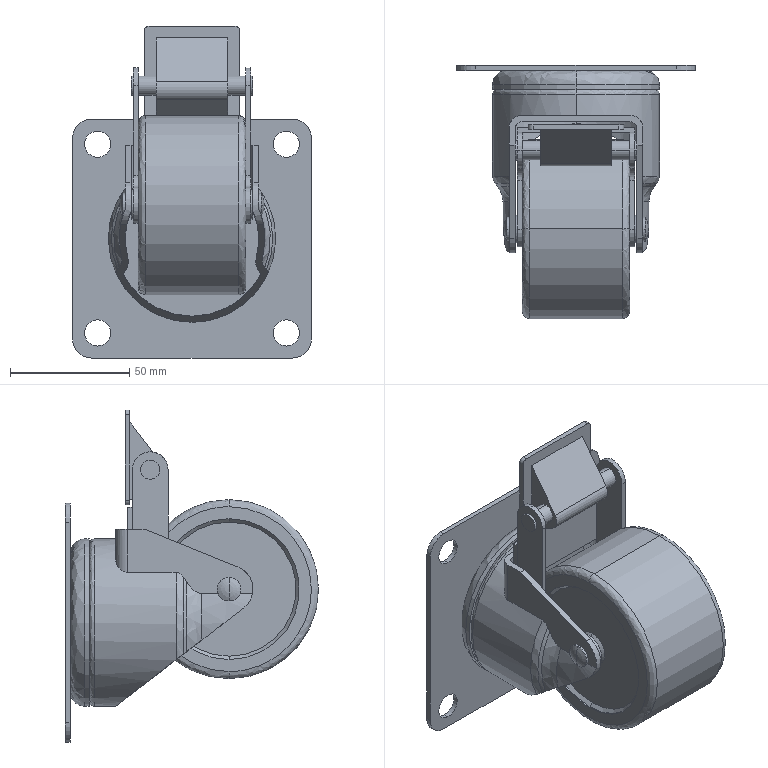Part | SolidWorks | features BaseBody 5 | 5 solids | 162 faces | box 100 x 106 x 139 mm | volume 279325 mm3 | cylinder 70 | plane 56 | spline 16 | cone 16 | torus 4 | commonest cylinder face diameters 10 x9 8 x8 11 x8 15 x5 4 x4 12 x4